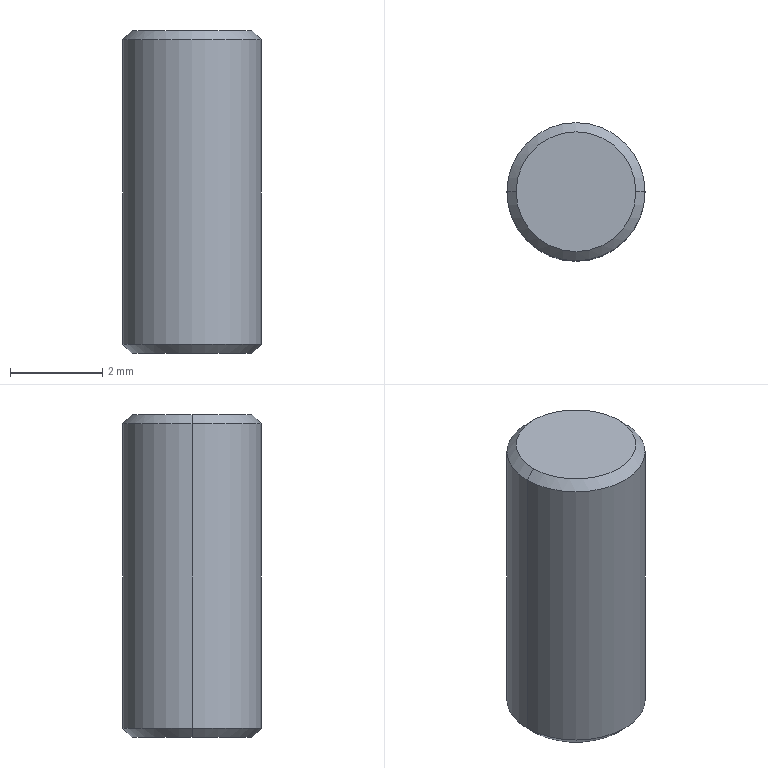Part | SolidWorks | features Chamfer 1, Extrusion 1 | 1 solid | 8 faces | box 3 x 3 x 7 mm | volume 49.12 mm3 | cone 4 | cylinder 2 | plane 2 | commonest cylinder face diameters 3 x2
STEP:
#1=CARTESIAN_POINT('',(-1.759,37.272,7.));
#2=VERTEX_POINT('',#1);
#3=CARTESIAN_POINT('',(-4.359,37.272,7.));
#4=VERTEX_POINT('',#3);
#5=CARTESIAN_POINT('',(-3.059,37.272,7.));
#6=DIRECTION('',(0.,0.,1.));
#7=DIRECTION('',(1.,0.,0.));
#8=AXIS2_PLACEMENT_3D('',#5,#6,#7);
#9=CIRCLE('',#8,1.3);
#10=EDGE_CURVE('',#2,#4,#9,.T.);
#11=ORIENTED_EDGE('',*,*,#10,.F.);
#12=CARTESIAN_POINT('',(-1.559,37.272,6.8));
#13=VERTEX_POINT('',#12);
#14=CARTESIAN_POINT('',(-1.759,37.272,7.));
#15=DIRECTION('',(0.7071,0.,-0.7071));
#16=VECTOR('',#15,1000.);
#17=LINE('',#14,#16);
#18=EDGE_CURVE('',#2,#13,#17,.T.);
#19=ORIENTED_EDGE('',*,*,#18,.T.);
#20=CARTESIAN_POINT('',(-4.559,37.272,6.8));
#21=VERTEX_POINT('',#20);
#22=CARTESIAN_POINT('',(-3.059,37.272,6.8));
#23=DIRECTION('',(0.,0.,-1.));
#24=DIRECTION('',(1.,0.,0.));
#25=AXIS2_PLACEMENT_3D('',#22,#23,#24);
#26=CIRCLE('',#25,1.5);
#27=EDGE_CURVE('',#21,#13,#26,.T.);
#28=ORIENTED_EDGE('',*,*,#27,.F.);
#29=CARTESIAN_POINT('',(-4.359,37.272,7.));
#30=DIRECTION('',(-0.7071,0.,-0.7071));
#31=VECTOR('',#30,1000.);
#32=LINE('',#29,#31);
#33=EDGE_CURVE('',#4,#21,#32,.T.);
#34=ORIENTED_EDGE('',*,*,#33,.F.);
#35=EDGE_LOOP('',(#11,#19,#28,#34));
#36=FACE_OUTER_BOUND('',#35,.T.);
#37=CARTESIAN_POINT('',(-3.059,37.272,7.));
#38=DIRECTION('',(0.,0.,-1.));
#39=DIRECTION('',(-1.,0.,0.));
#40=AXIS2_PLACEMENT_3D('',#37,#38,#39);
#41=CONICAL_SURFACE('',#40,1.3,0.7854);
#42=ADVANCED_FACE('',(#36),#41,.T.);
#43=CARTESIAN_POINT('',(-4.359,37.272,0.));
#44=VERTEX_POINT('',#43);
#45=CARTESIAN_POINT('',(-1.759,37.272,0.));
#46=VERTEX_POINT('',#45);
#47=CARTESIAN_POINT('',(-3.059,37.272,0.));
#48=DIRECTION('',(0.,0.,-1.));
#49=DIRECTION('',(1.,0.,0.));
#50=AXIS2_PLACEMENT_3D('',#47,#48,#49);
#51=CIRCLE('',#50,1.3);
#52=EDGE_CURVE('',#44,#46,#51,.T.);
#53=ORIENTED_EDGE('',*,*,#52,.F.);
#54=CARTESIAN_POINT('',(-4.559,37.272,0.2));
#55=VERTEX_POINT('',#54);
#56=CARTESIAN_POINT('',(-4.559,37.272,0.2));
#57=DIRECTION('',(-0.7071,0.,0.7071));
#58=VECTOR('',#57,1000.);
#59=LINE('',#56,#58);
#60=EDGE_CURVE('',#44,#55,#59,.T.);
#61=ORIENTED_EDGE('',*,*,#60,.T.);
#62=CARTESIAN_POINT('',(-1.559,37.272,0.2));
#63=VERTEX_POINT('',#62);
#64=CARTESIAN_POINT('',(-3.059,37.272,0.2));
#65=DIRECTION('',(0.,0.,1.));
#66=DIRECTION('',(1.,0.,0.));
#67=AXIS2_PLACEMENT_3D('',#64,#65,#66);
#68=CIRCLE('',#67,1.5);
#69=EDGE_CURVE('',#63,#55,#68,.T.);
#70=ORIENTED_EDGE('',*,*,#69,.F.);
#71=CARTESIAN_POINT('',(-1.559,37.272,0.2));
#72=DIRECTION('',(0.7071,0.,0.7071));
#73=VECTOR('',#72,1000.);
#74=LINE('',#71,#73);
#75=EDGE_CURVE('',#46,#63,#74,.T.);
#76=ORIENTED_EDGE('',*,*,#75,.F.);
#77=EDGE_LOOP('',(#53,#61,#70,#76));
#78=FACE_OUTER_BOUND('',#77,.T.);
#79=CARTESIAN_POINT('',(-3.059,37.272,0.2));
#80=DIRECTION('',(0.,0.,1.));
#81=DIRECTION('',(1.,0.,0.));
#82=AXIS2_PLACEMENT_3D('',#79,#80,#81);
#83=CONICAL_SURFACE('',#82,1.5,0.7854);
#84=ADVANCED_FACE('',(#78),#83,.T.);
#85=ORIENTED_EDGE('',*,*,#27,.T.);
#86=CARTESIAN_POINT('',(-1.559,37.272,7.));
#87=DIRECTION('',(0.,0.,-1.));
#88=VECTOR('',#87,1000.);
#89=LINE('',#86,#88);
#90=EDGE_CURVE('',#13,#63,#89,.T.);
#91=ORIENTED_EDGE('',*,*,#90,.T.);
#92=ORIENTED_EDGE('',*,*,#69,.T.);
#93=CARTESIAN_POINT('',(-4.559,37.272,7.));
#94=DIRECTION('',(0.,0.,-1.));
#95=VECTOR('',#94,1000.);
#96=LINE('',#93,#95);
#97=EDGE_CURVE('',#21,#55,#96,.T.);
#98=ORIENTED_EDGE('',*,*,#97,.F.);
#99=EDGE_LOOP('',(#85,#91,#92,#98));
#100=FACE_OUTER_BOUND('',#99,.T.);
#101=CARTESIAN_POINT('',(-3.059,37.272,7.));
#102=DIRECTION('',(0.,0.,-1.));
#103=DIRECTION('',(-1.,0.,0.));
#104=AXIS2_PLACEMENT_3D('',#101,#102,#103);
#105=CYLINDRICAL_SURFACE('',#104,1.5);
#106=ADVANCED_FACE('',(#100),#105,.T.);
#107=ORIENTED_EDGE('',*,*,#90,.F.);
#108=CARTESIAN_POINT('',(-3.059,37.272,6.8));
#109=DIRECTION('',(0.,0.,-1.));
#110=DIRECTION('',(1.,0.,0.));
#111=AXIS2_PLACEMENT_3D('',#108,#109,#110);
#112=CIRCLE('',#111,1.5);
#113=EDGE_CURVE('',#13,#21,#112,.T.);
#114=ORIENTED_EDGE('',*,*,#113,.T.);
#115=ORIENTED_EDGE('',*,*,#97,.T.);
#116=CARTESIAN_POINT('',(-3.059,37.272,0.2));
#117=DIRECTION('',(0.,0.,1.));
#118=DIRECTION('',(1.,0.,0.));
#119=AXIS2_PLACEMENT_3D('',#116,#117,#118);
#120=CIRCLE('',#119,1.5);
#121=EDGE_CURVE('',#55,#63,#120,.T.);
#122=ORIENTED_EDGE('',*,*,#121,.T.);
#123=EDGE_LOOP('',(#107,#114,#115,#122));
#124=FACE_OUTER_BOUND('',#123,.T.);
#125=CARTESIAN_POINT('',(-3.059,37.272,7.));
#126=DIRECTION('',(0.,0.,-1.));
#127=DIRECTION('',(-1.,0.,0.));
#128=AXIS2_PLACEMENT_3D('',#125,#126,#127);
#129=CYLINDRICAL_SURFACE('',#128,1.5);
#130=ADVANCED_FACE('',(#124),#129,.T.);
#131=CARTESIAN_POINT('',(-3.059,37.272,7.));
#132=DIRECTION('',(0.,0.,1.));
#133=DIRECTION('',(1.,0.,0.));
#134=AXIS2_PLACEMENT_3D('',#131,#132,#133);
#135=CIRCLE('',#134,1.3);
#136=EDGE_CURVE('',#4,#2,#135,.T.);
#137=ORIENTED_EDGE('',*,*,#136,.T.);
#138=ORIENTED_EDGE('',*,*,#10,.T.);
#139=EDGE_LOOP('',(#137,#138));
#140=FACE_OUTER_BOUND('',#139,.T.);
#141=CARTESIAN_POINT('',(-3.059,37.272,7.));
#142=DIRECTION('',(0.,0.,1.));
#143=DIRECTION('',(1.,0.,0.));
#144=AXIS2_PLACEMENT_3D('',#141,#142,#143);
#145=PLANE('',#144);
#146=ADVANCED_FACE('',(#140),#145,.T.);
#147=CARTESIAN_POINT('',(-3.059,37.272,0.));
#148=DIRECTION('',(0.,0.,-1.));
#149=DIRECTION('',(1.,0.,0.));
#150=AXIS2_PLACEMENT_3D('',#147,#148,#149);
#151=CIRCLE('',#150,1.3);
#152=EDGE_CURVE('',#46,#44,#151,.T.);
#153=ORIENTED_EDGE('',*,*,#152,.T.);
#154=ORIENTED_EDGE('',*,*,#52,.T.);
#155=EDGE_LOOP('',(#153,#154));
#156=FACE_OUTER_BOUND('',#155,.T.);
#157=CARTESIAN_POINT('',(-3.059,37.272,0.));
#158=DIRECTION('',(0.,0.,1.));
#159=DIRECTION('',(1.,0.,0.));
#160=AXIS2_PLACEMENT_3D('',#157,#158,#159);
#161=PLANE('',#160);
#162=ADVANCED_FACE('',(#156),#161,.F.);
#163=ORIENTED_EDGE('',*,*,#60,.F.);
#164=ORIENTED_EDGE('',*,*,#152,.F.);
#165=ORIENTED_EDGE('',*,*,#75,.T.);
#166=ORIENTED_EDGE('',*,*,#121,.F.);
#167=EDGE_LOOP('',(#163,#164,#165,#166));
#168=FACE_OUTER_BOUND('',#167,.T.);
#169=CARTESIAN_POINT('',(-3.059,37.272,0.2));
#170=DIRECTION('',(0.,0.,1.));
#171=DIRECTION('',(1.,0.,0.));
#172=AXIS2_PLACEMENT_3D('',#169,#170,#171);
#173=CONICAL_SURFACE('',#172,1.5,0.7854);
#174=ADVANCED_FACE('',(#168),#173,.T.);
#175=ORIENTED_EDGE('',*,*,#18,.F.);
#176=ORIENTED_EDGE('',*,*,#136,.F.);
#177=ORIENTED_EDGE('',*,*,#33,.T.);
#178=ORIENTED_EDGE('',*,*,#113,.F.);
#179=EDGE_LOOP('',(#175,#176,#177,#178));
#180=FACE_OUTER_BOUND('',#179,.T.);
#181=CARTESIAN_POINT('',(-3.059,37.272,7.));
#182=DIRECTION('',(0.,0.,-1.));
#183=DIRECTION('',(-1.,0.,0.));
#184=AXIS2_PLACEMENT_3D('',#181,#182,#183);
#185=CONICAL_SURFACE('',#184,1.3,0.7854);
#186=ADVANCED_FACE('',(#180),#185,.T.);
#187=CLOSED_SHELL('',(#42,#84,#106,#130,#146,#162,#174,#186));
#188=MANIFOLD_SOLID_BREP('',#187);
#189=CARTESIAN_POINT('',(0.,0.,0.));
#190=DIRECTION('',(0.,0.,1.));
#191=DIRECTION('',(1.,0.,0.));
#192=AXIS2_PLACEMENT_3D('',#189,#190,#191);
#193=(LENGTH_UNIT()NAMED_UNIT(*)SI_UNIT(.MILLI.,.METRE.));
#194=UNCERTAINTY_MEASURE_WITH_UNIT(LENGTH_MEASURE(0.00001),#193,'','');
#195=(NAMED_UNIT(*)PLANE_ANGLE_UNIT()SI_UNIT($,.RADIAN.));
#196=(NAMED_UNIT(*)SI_UNIT($,.STERADIAN.)SOLID_ANGLE_UNIT());
#197=(GEOMETRIC_REPRESENTATION_CONTEXT(3)GLOBAL_UNCERTAINTY_ASSIGNED_CONTEXT((#194))GLOBAL_UNIT_ASSIGNED_CONTEXT((#193,#195,#196))REPRESENTATION_CONTEXT('',''));
#198=ADVANCED_BREP_SHAPE_REPRESENTATION('',(#188,#192),#197);